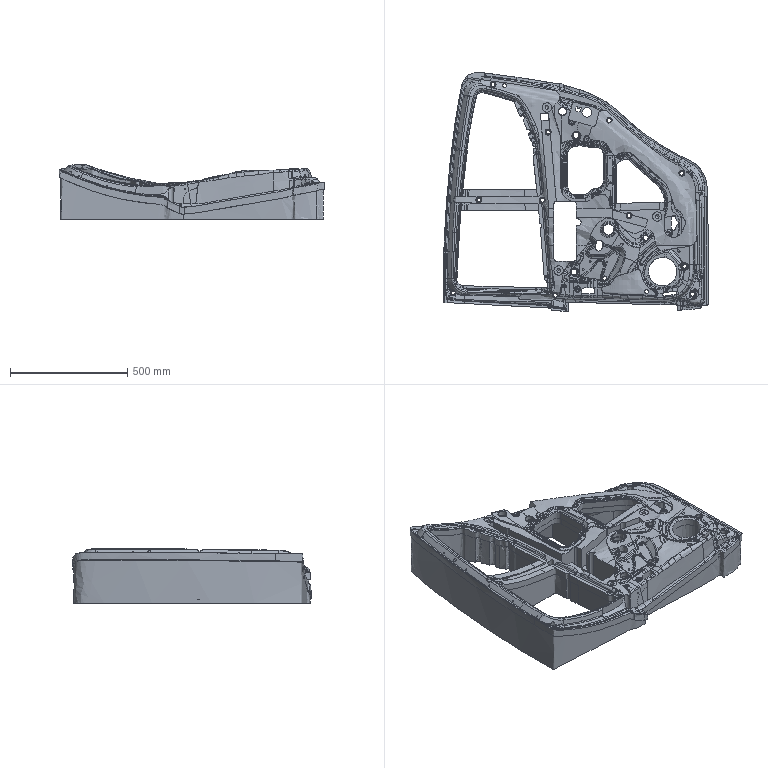Part | NX | features solid 2 | 1 solid | 1904 faces | box 1130 x 1018 x 233.961 mm | volume 89711219 mm3 | spline 1701 | plane 103 | cylinder 93 | sphere 4 | cone 3 | commonest cylinder face diameters 20 x11 17 x10 26 x10 25 x8 16 x7 60 x6